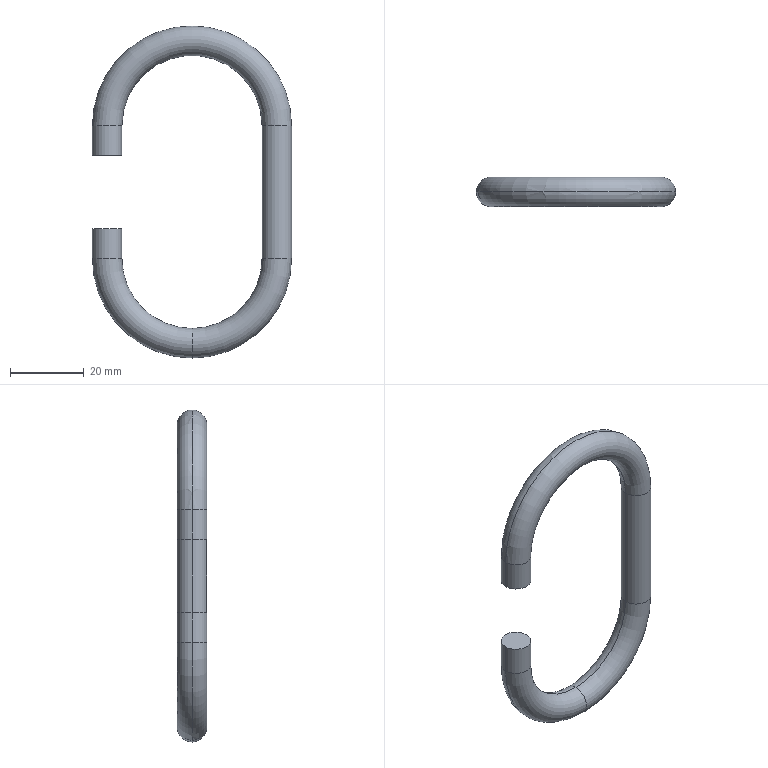Part | SolidWorks | features Sweep 1 | 1 solid | 14 faces | box 54 x 8 x 90 mm | volume 9878 mm3 | torus 6 | cylinder 6 | plane 2 | commonest cylinder face diameters 8 x6
STEP:
#1=CARTESIAN_POINT('',(0.,0.,-45.));
#2=VERTEX_POINT('',#1);
#3=CARTESIAN_POINT('',(0.,0.,-37.));
#4=VERTEX_POINT('',#3);
#5=CARTESIAN_POINT('',(0.,0.,-41.));
#6=DIRECTION('',(-1.,0.,0.));
#7=DIRECTION('',(0.,0.,1.));
#8=AXIS2_PLACEMENT_3D('',#5,#6,#7);
#9=CIRCLE('',#8,4.);
#10=EDGE_CURVE('',#2,#4,#9,.T.);
#11=ORIENTED_EDGE('',*,*,#10,.F.);
#12=CARTESIAN_POINT('',(27.,0.,-18.));
#13=VERTEX_POINT('',#12);
#14=CARTESIAN_POINT('',(0.,0.,-18.));
#15=DIRECTION('',(0.,-1.,0.));
#16=DIRECTION('',(0.,0.,-1.));
#17=AXIS2_PLACEMENT_3D('',#14,#15,#16);
#18=CIRCLE('',#17,27.);
#19=EDGE_CURVE('',#2,#13,#18,.T.);
#20=ORIENTED_EDGE('',*,*,#19,.T.);
#21=CARTESIAN_POINT('',(19.,0.,-18.));
#22=VERTEX_POINT('',#21);
#23=CARTESIAN_POINT('',(23.,0.,-18.));
#24=DIRECTION('',(0.,0.,-1.));
#25=DIRECTION('',(-1.,0.,0.));
#26=AXIS2_PLACEMENT_3D('',#23,#24,#25);
#27=CIRCLE('',#26,4.);
#28=EDGE_CURVE('',#13,#22,#27,.T.);
#29=ORIENTED_EDGE('',*,*,#28,.T.);
#30=CARTESIAN_POINT('',(0.,0.,-18.));
#31=DIRECTION('',(0.,-1.,0.));
#32=DIRECTION('',(0.,0.,-1.));
#33=AXIS2_PLACEMENT_3D('',#30,#31,#32);
#34=CIRCLE('',#33,19.);
#35=EDGE_CURVE('',#4,#22,#34,.T.);
#36=ORIENTED_EDGE('',*,*,#35,.F.);
#37=EDGE_LOOP('',(#11,#20,#29,#36));
#38=FACE_OUTER_BOUND('',#37,.T.);
#39=CARTESIAN_POINT('',(0.,0.,-18.));
#40=DIRECTION('',(0.,-1.,0.));
#41=DIRECTION('',(0.,0.,-1.));
#42=AXIS2_PLACEMENT_3D('',#39,#40,#41);
#43=TOROIDAL_SURFACE('',#42,23.,4.);
#44=ADVANCED_FACE('',(#38),#43,.T.);
#45=CARTESIAN_POINT('',(27.,0.,18.));
#46=VERTEX_POINT('',#45);
#47=CARTESIAN_POINT('',(19.,0.,18.));
#48=VERTEX_POINT('',#47);
#49=CARTESIAN_POINT('',(23.,0.,18.));
#50=DIRECTION('',(0.,0.,-1.));
#51=DIRECTION('',(-1.,0.,0.));
#52=AXIS2_PLACEMENT_3D('',#49,#50,#51);
#53=CIRCLE('',#52,4.);
#54=EDGE_CURVE('',#46,#48,#53,.T.);
#55=ORIENTED_EDGE('',*,*,#54,.F.);
#56=CARTESIAN_POINT('',(-27.,0.,18.));
#57=VERTEX_POINT('',#56);
#58=CARTESIAN_POINT('',(0.,0.,18.));
#59=DIRECTION('',(0.,-1.,0.));
#60=DIRECTION('',(0.,0.,-1.));
#61=AXIS2_PLACEMENT_3D('',#58,#59,#60);
#62=CIRCLE('',#61,27.);
#63=EDGE_CURVE('',#46,#57,#62,.T.);
#64=ORIENTED_EDGE('',*,*,#63,.T.);
#65=CARTESIAN_POINT('',(-19.,0.,18.));
#66=VERTEX_POINT('',#65);
#67=CARTESIAN_POINT('',(-23.,0.,18.));
#68=DIRECTION('',(0.,0.,1.));
#69=DIRECTION('',(1.,0.,0.));
#70=AXIS2_PLACEMENT_3D('',#67,#68,#69);
#71=CIRCLE('',#70,4.);
#72=EDGE_CURVE('',#57,#66,#71,.T.);
#73=ORIENTED_EDGE('',*,*,#72,.T.);
#74=CARTESIAN_POINT('',(0.,0.,18.));
#75=DIRECTION('',(0.,-1.,0.));
#76=DIRECTION('',(0.,0.,-1.));
#77=AXIS2_PLACEMENT_3D('',#74,#75,#76);
#78=CIRCLE('',#77,19.);
#79=EDGE_CURVE('',#48,#66,#78,.T.);
#80=ORIENTED_EDGE('',*,*,#79,.F.);
#81=EDGE_LOOP('',(#55,#64,#73,#80));
#82=FACE_OUTER_BOUND('',#81,.T.);
#83=CARTESIAN_POINT('',(0.,0.,18.));
#84=DIRECTION('',(0.,-1.,0.));
#85=DIRECTION('',(0.,0.,-1.));
#86=AXIS2_PLACEMENT_3D('',#83,#84,#85);
#87=TOROIDAL_SURFACE('',#86,23.,4.);
#88=ADVANCED_FACE('',(#82),#87,.T.);
#89=CARTESIAN_POINT('',(-27.,0.,-18.));
#90=VERTEX_POINT('',#89);
#91=CARTESIAN_POINT('',(-19.,0.,-18.));
#92=VERTEX_POINT('',#91);
#93=CARTESIAN_POINT('',(-23.,0.,-18.));
#94=DIRECTION('',(0.,0.,1.));
#95=DIRECTION('',(1.,0.,0.));
#96=AXIS2_PLACEMENT_3D('',#93,#94,#95);
#97=CIRCLE('',#96,4.);
#98=EDGE_CURVE('',#90,#92,#97,.T.);
#99=ORIENTED_EDGE('',*,*,#98,.F.);
#100=CARTESIAN_POINT('',(0.,0.,-18.));
#101=DIRECTION('',(0.,-1.,0.));
#102=DIRECTION('',(0.,0.,-1.));
#103=AXIS2_PLACEMENT_3D('',#100,#101,#102);
#104=CIRCLE('',#103,27.);
#105=EDGE_CURVE('',#90,#2,#104,.T.);
#106=ORIENTED_EDGE('',*,*,#105,.T.);
#107=ORIENTED_EDGE('',*,*,#10,.T.);
#108=CARTESIAN_POINT('',(0.,0.,-18.));
#109=DIRECTION('',(0.,-1.,0.));
#110=DIRECTION('',(0.,0.,-1.));
#111=AXIS2_PLACEMENT_3D('',#108,#109,#110);
#112=CIRCLE('',#111,19.);
#113=EDGE_CURVE('',#92,#4,#112,.T.);
#114=ORIENTED_EDGE('',*,*,#113,.F.);
#115=EDGE_LOOP('',(#99,#106,#107,#114));
#116=FACE_OUTER_BOUND('',#115,.T.);
#117=CARTESIAN_POINT('',(0.,0.,-18.));
#118=DIRECTION('',(0.,-1.,0.));
#119=DIRECTION('',(0.,0.,-1.));
#120=AXIS2_PLACEMENT_3D('',#117,#118,#119);
#121=TOROIDAL_SURFACE('',#120,23.,4.);
#122=ADVANCED_FACE('',(#116),#121,.T.);
#123=CARTESIAN_POINT('',(-23.,0.,-18.));
#124=DIRECTION('',(0.,0.,1.));
#125=DIRECTION('',(1.,0.,0.));
#126=AXIS2_PLACEMENT_3D('',#123,#124,#125);
#127=CIRCLE('',#126,4.);
#128=EDGE_CURVE('',#92,#90,#127,.T.);
#129=ORIENTED_EDGE('',*,*,#128,.T.);
#130=CARTESIAN_POINT('',(-27.,0.,-10.));
#131=VERTEX_POINT('',#130);
#132=CARTESIAN_POINT('',(-27.,0.,-18.));
#133=DIRECTION('',(0.,0.,1.));
#134=VECTOR('',#133,1000.);
#135=LINE('',#132,#134);
#136=EDGE_CURVE('',#90,#131,#135,.T.);
#137=ORIENTED_EDGE('',*,*,#136,.T.);
#138=CARTESIAN_POINT('',(-19.,0.,-10.));
#139=VERTEX_POINT('',#138);
#140=CARTESIAN_POINT('',(-23.,0.,-10.));
#141=DIRECTION('',(0.,0.,1.));
#142=DIRECTION('',(1.,0.,0.));
#143=AXIS2_PLACEMENT_3D('',#140,#141,#142);
#144=CIRCLE('',#143,4.);
#145=EDGE_CURVE('',#139,#131,#144,.T.);
#146=ORIENTED_EDGE('',*,*,#145,.F.);
#147=CARTESIAN_POINT('',(-19.,0.,-18.));
#148=DIRECTION('',(0.,0.,1.));
#149=VECTOR('',#148,1000.);
#150=LINE('',#147,#149);
#151=EDGE_CURVE('',#92,#139,#150,.T.);
#152=ORIENTED_EDGE('',*,*,#151,.F.);
#153=EDGE_LOOP('',(#129,#137,#146,#152));
#154=FACE_OUTER_BOUND('',#153,.T.);
#155=CARTESIAN_POINT('',(-23.,0.,-18.));
#156=DIRECTION('',(0.,0.,1.));
#157=DIRECTION('',(1.,0.,0.));
#158=AXIS2_PLACEMENT_3D('',#155,#156,#157);
#159=CYLINDRICAL_SURFACE('',#158,4.);
#160=ADVANCED_FACE('',(#154),#159,.T.);
#161=ORIENTED_EDGE('',*,*,#105,.F.);
#162=ORIENTED_EDGE('',*,*,#128,.F.);
#163=ORIENTED_EDGE('',*,*,#113,.T.);
#164=CARTESIAN_POINT('',(0.,0.,-41.));
#165=DIRECTION('',(-1.,0.,0.));
#166=DIRECTION('',(0.,0.,1.));
#167=AXIS2_PLACEMENT_3D('',#164,#165,#166);
#168=CIRCLE('',#167,4.);
#169=EDGE_CURVE('',#4,#2,#168,.T.);
#170=ORIENTED_EDGE('',*,*,#169,.T.);
#171=EDGE_LOOP('',(#161,#162,#163,#170));
#172=FACE_OUTER_BOUND('',#171,.T.);
#173=CARTESIAN_POINT('',(0.,0.,-18.));
#174=DIRECTION('',(0.,-1.,0.));
#175=DIRECTION('',(0.,0.,-1.));
#176=AXIS2_PLACEMENT_3D('',#173,#174,#175);
#177=TOROIDAL_SURFACE('',#176,23.,4.);
#178=ADVANCED_FACE('',(#172),#177,.T.);
#179=CARTESIAN_POINT('',(23.,0.,-18.));
#180=DIRECTION('',(0.,0.,-1.));
#181=DIRECTION('',(-1.,0.,0.));
#182=AXIS2_PLACEMENT_3D('',#179,#180,#181);
#183=CIRCLE('',#182,4.);
#184=EDGE_CURVE('',#22,#13,#183,.T.);
#185=ORIENTED_EDGE('',*,*,#184,.F.);
#186=CARTESIAN_POINT('',(19.,0.,-18.));
#187=DIRECTION('',(0.,0.,1.));
#188=VECTOR('',#187,1000.);
#189=LINE('',#186,#188);
#190=EDGE_CURVE('',#22,#48,#189,.T.);
#191=ORIENTED_EDGE('',*,*,#190,.T.);
#192=CARTESIAN_POINT('',(23.,0.,18.));
#193=DIRECTION('',(0.,0.,-1.));
#194=DIRECTION('',(-1.,0.,0.));
#195=AXIS2_PLACEMENT_3D('',#192,#193,#194);
#196=CIRCLE('',#195,4.);
#197=EDGE_CURVE('',#48,#46,#196,.T.);
#198=ORIENTED_EDGE('',*,*,#197,.T.);
#199=CARTESIAN_POINT('',(27.,0.,-18.));
#200=DIRECTION('',(0.,0.,1.));
#201=VECTOR('',#200,1000.);
#202=LINE('',#199,#201);
#203=EDGE_CURVE('',#13,#46,#202,.T.);
#204=ORIENTED_EDGE('',*,*,#203,.F.);
#205=EDGE_LOOP('',(#185,#191,#198,#204));
#206=FACE_OUTER_BOUND('',#205,.T.);
#207=CARTESIAN_POINT('',(23.,0.,-18.));
#208=DIRECTION('',(0.,0.,1.));
#209=DIRECTION('',(1.,0.,0.));
#210=AXIS2_PLACEMENT_3D('',#207,#208,#209);
#211=CYLINDRICAL_SURFACE('',#210,4.);
#212=ADVANCED_FACE('',(#206),#211,.T.);
#213=CARTESIAN_POINT('',(-23.,0.,18.));
#214=DIRECTION('',(0.,0.,1.));
#215=DIRECTION('',(1.,0.,0.));
#216=AXIS2_PLACEMENT_3D('',#213,#214,#215);
#217=CIRCLE('',#216,4.);
#218=EDGE_CURVE('',#66,#57,#217,.T.);
#219=ORIENTED_EDGE('',*,*,#218,.F.);
#220=CARTESIAN_POINT('',(-19.,0.,10.));
#221=VERTEX_POINT('',#220);
#222=CARTESIAN_POINT('',(-19.,0.,18.));
#223=DIRECTION('',(0.,0.,-1.));
#224=VECTOR('',#223,1000.);
#225=LINE('',#222,#224);
#226=EDGE_CURVE('',#66,#221,#225,.T.);
#227=ORIENTED_EDGE('',*,*,#226,.T.);
#228=CARTESIAN_POINT('',(-27.,0.,10.));
#229=VERTEX_POINT('',#228);
#230=CARTESIAN_POINT('',(-23.,0.,10.));
#231=DIRECTION('',(0.,0.,1.));
#232=DIRECTION('',(1.,0.,0.));
#233=AXIS2_PLACEMENT_3D('',#230,#231,#232);
#234=CIRCLE('',#233,4.);
#235=EDGE_CURVE('',#221,#229,#234,.T.);
#236=ORIENTED_EDGE('',*,*,#235,.T.);
#237=CARTESIAN_POINT('',(-27.,0.,18.));
#238=DIRECTION('',(0.,0.,-1.));
#239=VECTOR('',#238,1000.);
#240=LINE('',#237,#239);
#241=EDGE_CURVE('',#57,#229,#240,.T.);
#242=ORIENTED_EDGE('',*,*,#241,.F.);
#243=EDGE_LOOP('',(#219,#227,#236,#242));
#244=FACE_OUTER_BOUND('',#243,.T.);
#245=CARTESIAN_POINT('',(-23.,0.,18.));
#246=DIRECTION('',(0.,0.,-1.));
#247=DIRECTION('',(-1.,0.,0.));
#248=AXIS2_PLACEMENT_3D('',#245,#246,#247);
#249=CYLINDRICAL_SURFACE('',#248,4.);
#250=ADVANCED_FACE('',(#244),#249,.T.);
#251=ORIENTED_EDGE('',*,*,#226,.F.);
#252=ORIENTED_EDGE('',*,*,#72,.F.);
#253=ORIENTED_EDGE('',*,*,#241,.T.);
#254=CARTESIAN_POINT('',(-23.,0.,10.));
#255=DIRECTION('',(0.,0.,1.));
#256=DIRECTION('',(1.,0.,0.));
#257=AXIS2_PLACEMENT_3D('',#254,#255,#256);
#258=CIRCLE('',#257,4.);
#259=EDGE_CURVE('',#229,#221,#258,.T.);
#260=ORIENTED_EDGE('',*,*,#259,.T.);
#261=EDGE_LOOP('',(#251,#252,#253,#260));
#262=FACE_OUTER_BOUND('',#261,.T.);
#263=CARTESIAN_POINT('',(-23.,0.,18.));
#264=DIRECTION('',(0.,0.,-1.));
#265=DIRECTION('',(-1.,0.,0.));
#266=AXIS2_PLACEMENT_3D('',#263,#264,#265);
#267=CYLINDRICAL_SURFACE('',#266,4.);
#268=ADVANCED_FACE('',(#262),#267,.T.);
#269=ORIENTED_EDGE('',*,*,#63,.F.);
#270=ORIENTED_EDGE('',*,*,#197,.F.);
#271=ORIENTED_EDGE('',*,*,#79,.T.);
#272=ORIENTED_EDGE('',*,*,#218,.T.);
#273=EDGE_LOOP('',(#269,#270,#271,#272));
#274=FACE_OUTER_BOUND('',#273,.T.);
#275=CARTESIAN_POINT('',(0.,0.,18.));
#276=DIRECTION('',(0.,-1.,0.));
#277=DIRECTION('',(0.,0.,-1.));
#278=AXIS2_PLACEMENT_3D('',#275,#276,#277);
#279=TOROIDAL_SURFACE('',#278,23.,4.);
#280=ADVANCED_FACE('',(#274),#279,.T.);
#281=ORIENTED_EDGE('',*,*,#190,.F.);
#282=ORIENTED_EDGE('',*,*,#28,.F.);
#283=ORIENTED_EDGE('',*,*,#203,.T.);
#284=ORIENTED_EDGE('',*,*,#54,.T.);
#285=EDGE_LOOP('',(#281,#282,#283,#284));
#286=FACE_OUTER_BOUND('',#285,.T.);
#287=CARTESIAN_POINT('',(23.,0.,-18.));
#288=DIRECTION('',(0.,0.,1.));
#289=DIRECTION('',(1.,0.,0.));
#290=AXIS2_PLACEMENT_3D('',#287,#288,#289);
#291=CYLINDRICAL_SURFACE('',#290,4.);
#292=ADVANCED_FACE('',(#286),#291,.T.);
#293=ORIENTED_EDGE('',*,*,#19,.F.);
#294=ORIENTED_EDGE('',*,*,#169,.F.);
#295=ORIENTED_EDGE('',*,*,#35,.T.);
#296=ORIENTED_EDGE('',*,*,#184,.T.);
#297=EDGE_LOOP('',(#293,#294,#295,#296));
#298=FACE_OUTER_BOUND('',#297,.T.);
#299=CARTESIAN_POINT('',(0.,0.,-18.));
#300=DIRECTION('',(0.,-1.,0.));
#301=DIRECTION('',(0.,0.,-1.));
#302=AXIS2_PLACEMENT_3D('',#299,#300,#301);
#303=TOROIDAL_SURFACE('',#302,23.,4.);
#304=ADVANCED_FACE('',(#298),#303,.T.);
#305=ORIENTED_EDGE('',*,*,#136,.F.);
#306=ORIENTED_EDGE('',*,*,#98,.T.);
#307=ORIENTED_EDGE('',*,*,#151,.T.);
#308=CARTESIAN_POINT('',(-23.,0.,-10.));
#309=DIRECTION('',(0.,0.,1.));
#310=DIRECTION('',(1.,0.,0.));
#311=AXIS2_PLACEMENT_3D('',#308,#309,#310);
#312=CIRCLE('',#311,4.);
#313=EDGE_CURVE('',#131,#139,#312,.T.);
#314=ORIENTED_EDGE('',*,*,#313,.F.);
#315=EDGE_LOOP('',(#305,#306,#307,#314));
#316=FACE_OUTER_BOUND('',#315,.T.);
#317=CARTESIAN_POINT('',(-23.,0.,-18.));
#318=DIRECTION('',(0.,0.,1.));
#319=DIRECTION('',(1.,0.,0.));
#320=AXIS2_PLACEMENT_3D('',#317,#318,#319);
#321=CYLINDRICAL_SURFACE('',#320,4.);
#322=ADVANCED_FACE('',(#316),#321,.T.);
#323=ORIENTED_EDGE('',*,*,#259,.F.);
#324=ORIENTED_EDGE('',*,*,#235,.F.);
#325=EDGE_LOOP('',(#323,#324));
#326=FACE_OUTER_BOUND('',#325,.T.);
#327=CARTESIAN_POINT('',(-23.,0.,10.));
#328=DIRECTION('',(0.,0.,1.));
#329=DIRECTION('',(1.,0.,0.));
#330=AXIS2_PLACEMENT_3D('',#327,#328,#329);
#331=PLANE('',#330);
#332=ADVANCED_FACE('',(#326),#331,.F.);
#333=ORIENTED_EDGE('',*,*,#145,.T.);
#334=ORIENTED_EDGE('',*,*,#313,.T.);
#335=EDGE_LOOP('',(#333,#334));
#336=FACE_OUTER_BOUND('',#335,.T.);
#337=CARTESIAN_POINT('',(-23.,0.,-10.));
#338=DIRECTION('',(0.,0.,1.));
#339=DIRECTION('',(1.,0.,0.));
#340=AXIS2_PLACEMENT_3D('',#337,#338,#339);
#341=PLANE('',#340);
#342=ADVANCED_FACE('',(#336),#341,.T.);
#343=CLOSED_SHELL('',(#44,#88,#122,#160,#178,#212,#250,#268,#280,#292,#304,#322,#332,#342));
#344=MANIFOLD_SOLID_BREP('',#343);
#345=CARTESIAN_POINT('',(0.,0.,0.));
#346=DIRECTION('',(0.,0.,1.));
#347=DIRECTION('',(1.,0.,0.));
#348=AXIS2_PLACEMENT_3D('',#345,#346,#347);
#349=(LENGTH_UNIT()NAMED_UNIT(*)SI_UNIT(.MILLI.,.METRE.));
#350=UNCERTAINTY_MEASURE_WITH_UNIT(LENGTH_MEASURE(0.00001),#349,'','');
#351=(NAMED_UNIT(*)PLANE_ANGLE_UNIT()SI_UNIT($,.RADIAN.));
#352=(NAMED_UNIT(*)SI_UNIT($,.STERADIAN.)SOLID_ANGLE_UNIT());
#353=(GEOMETRIC_REPRESENTATION_CONTEXT(3)GLOBAL_UNCERTAINTY_ASSIGNED_CONTEXT((#350))GLOBAL_UNIT_ASSIGNED_CONTEXT((#349,#351,#352))REPRESENTATION_CONTEXT('',''));
#354=ADVANCED_BREP_SHAPE_REPRESENTATION('',(#344,#348),#353);